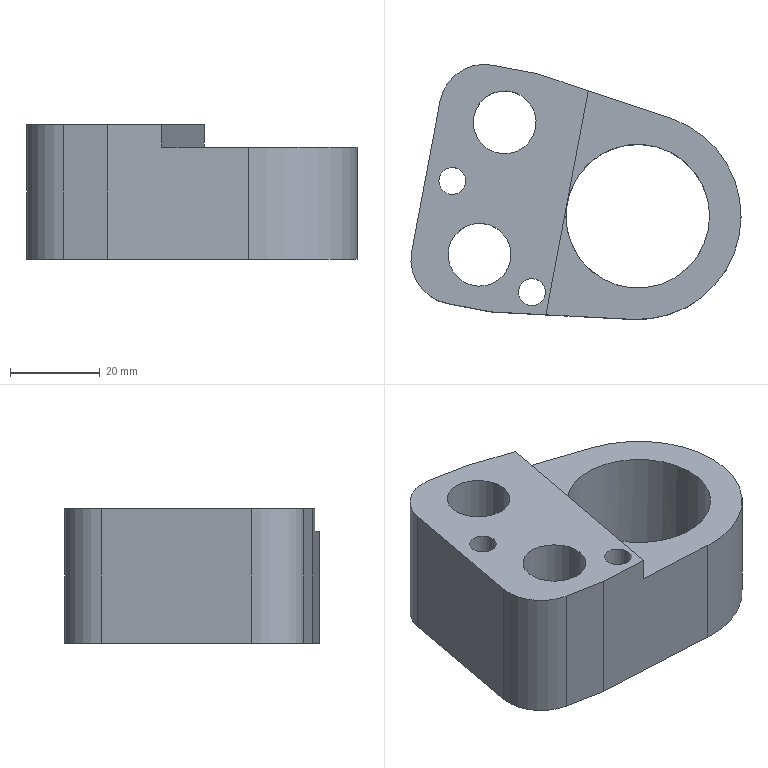Part | NX | features solid 2 | 1 solid | 25 faces | box 73.499 x 56.771 x 30 mm | volume 54639 mm3 | plane 13 | cylinder 12 | commonest cylinder face diameters 6 x2 8 x2 14 x2 19 x2 20 x2 32 x1
STEP:
#1=CARTESIAN_POINT('',(-713.065,445.332,68.));
#2=VERTEX_POINT('',#1);
#3=CARTESIAN_POINT('',(-716.996,446.076,68.));
#4=DIRECTION('',(0.,0.,1.));
#5=DIRECTION('',(0.9826,-0.186,0.));
#6=AXIS2_PLACEMENT_3D('',#3,#4,#5);
#7=CIRCLE('',#6,4.);
#8=EDGE_CURVE('',#2,#2,#7,.F.);
#9=ORIENTED_EDGE('',*,*,#8,.F.);
#10=EDGE_LOOP('',(#9));
#11=FACE_BOUND('',#10,.T.);
#12=CARTESIAN_POINT('',(-720.277,431.431,68.));
#13=VERTEX_POINT('',#12);
#14=CARTESIAN_POINT('',(-710.942,429.664,68.));
#15=DIRECTION('',(0.,0.,-1.));
#16=DIRECTION('',(-0.9826,0.186,0.));
#17=AXIS2_PLACEMENT_3D('',#14,#15,#16);
#18=CIRCLE('',#17,9.5);
#19=EDGE_CURVE('',#13,#13,#18,.T.);
#20=ORIENTED_EDGE('',*,*,#19,.F.);
#21=EDGE_LOOP('',(#20));
#22=FACE_BOUND('',#21,.T.);
#23=CARTESIAN_POINT('',(-714.697,460.908,68.));
#24=VERTEX_POINT('',#23);
#25=CARTESIAN_POINT('',(-705.363,459.141,68.));
#26=DIRECTION('',(0.,0.,-1.));
#27=DIRECTION('',(-0.9826,0.186,0.));
#28=AXIS2_PLACEMENT_3D('',#25,#26,#27);
#29=CIRCLE('',#28,9.5);
#30=EDGE_CURVE('',#24,#24,#29,.T.);
#31=ORIENTED_EDGE('',*,*,#30,.F.);
#32=EDGE_LOOP('',(#31));
#33=FACE_BOUND('',#32,.T.);
#34=CARTESIAN_POINT('',(-660.007,435.289,68.));
#35=VERTEX_POINT('',#34);
#36=CARTESIAN_POINT('',(-675.728,438.265,68.));
#37=DIRECTION('',(0.,0.,1.));
#38=DIRECTION('',(0.9826,-0.186,0.));
#39=AXIS2_PLACEMENT_3D('',#36,#37,#38);
#40=CIRCLE('',#39,16.);
#41=EDGE_CURVE('',#35,#35,#40,.T.);
#42=ORIENTED_EDGE('',*,*,#41,.T.);
#43=EDGE_LOOP('',(#42));
#44=FACE_BOUND('',#43,.T.);
#45=CARTESIAN_POINT('',(-668.458,460.086,68.));
#46=VERTEX_POINT('',#45);
#47=CARTESIAN_POINT('',(-698.218,470.002,68.));
#48=VERTEX_POINT('',#47);
#49=CARTESIAN_POINT('',(-668.458,460.086,68.));
#50=DIRECTION('',(-0.9487,0.3161,0.));
#51=VECTOR('',#50,1000.);
#52=LINE('',#49,#51);
#53=EDGE_CURVE('',#46,#48,#52,.T.);
#54=ORIENTED_EDGE('',*,*,#53,.F.);
#55=CARTESIAN_POINT('',(-676.936,415.297,68.));
#56=VERTEX_POINT('',#55);
#57=CARTESIAN_POINT('',(-675.728,438.265,68.));
#58=DIRECTION('',(0.,0.,-1.));
#59=DIRECTION('',(-0.9826,0.186,0.));
#60=AXIS2_PLACEMENT_3D('',#57,#58,#59);
#61=CIRCLE('',#60,23.);
#62=EDGE_CURVE('',#46,#56,#61,.T.);
#63=ORIENTED_EDGE('',*,*,#62,.T.);
#64=CARTESIAN_POINT('',(-708.261,416.944,68.));
#65=VERTEX_POINT('',#64);
#66=CARTESIAN_POINT('',(-676.936,415.297,68.));
#67=DIRECTION('',(-0.9986,0.0525,0.));
#68=VECTOR('',#67,1000.);
#69=LINE('',#66,#68);
#70=EDGE_CURVE('',#56,#65,#69,.T.);
#71=ORIENTED_EDGE('',*,*,#70,.T.);
#72=CARTESIAN_POINT('',(-718.087,418.804,68.));
#73=VERTEX_POINT('',#72);
#74=CARTESIAN_POINT('',(-708.261,416.944,68.));
#75=DIRECTION('',(-0.9826,0.186,0.));
#76=VECTOR('',#75,1000.);
#77=LINE('',#74,#76);
#78=EDGE_CURVE('',#65,#73,#77,.T.);
#79=ORIENTED_EDGE('',*,*,#78,.T.);
#80=CARTESIAN_POINT('',(-726.053,430.489,68.));
#81=VERTEX_POINT('',#80);
#82=CARTESIAN_POINT('',(-716.227,428.629,68.));
#83=DIRECTION('',(0.,0.,-1.));
#84=DIRECTION('',(-0.9826,0.186,0.));
#85=AXIS2_PLACEMENT_3D('',#82,#83,#84);
#86=CIRCLE('',#85,10.);
#87=EDGE_CURVE('',#73,#81,#86,.T.);
#88=ORIENTED_EDGE('',*,*,#87,.T.);
#89=CARTESIAN_POINT('',(-719.729,463.896,68.));
#90=VERTEX_POINT('',#89);
#91=CARTESIAN_POINT('',(-719.729,463.896,68.));
#92=DIRECTION('',(-0.186,-0.9826,0.));
#93=VECTOR('',#92,1000.);
#94=LINE('',#91,#93);
#95=EDGE_CURVE('',#90,#81,#94,.T.);
#96=ORIENTED_EDGE('',*,*,#95,.F.);
#97=CARTESIAN_POINT('',(-708.044,471.861,68.));
#98=VERTEX_POINT('',#97);
#99=CARTESIAN_POINT('',(-709.904,462.036,68.));
#100=DIRECTION('',(0.,0.,-1.));
#101=DIRECTION('',(-0.9826,0.186,0.));
#102=AXIS2_PLACEMENT_3D('',#99,#100,#101);
#103=CIRCLE('',#102,10.);
#104=EDGE_CURVE('',#90,#98,#103,.T.);
#105=ORIENTED_EDGE('',*,*,#104,.T.);
#106=CARTESIAN_POINT('',(-698.218,470.002,68.));
#107=DIRECTION('',(-0.9826,0.186,0.));
#108=VECTOR('',#107,1000.);
#109=LINE('',#106,#108);
#110=EDGE_CURVE('',#48,#98,#109,.T.);
#111=ORIENTED_EDGE('',*,*,#110,.F.);
#112=EDGE_LOOP('',(#54,#63,#71,#79,#88,#96,#105,#111));
#113=FACE_BOUND('',#112,.T.);
#114=CARTESIAN_POINT('',(-695.355,420.607,68.));
#115=VERTEX_POINT('',#114);
#116=CARTESIAN_POINT('',(-699.285,421.351,68.));
#117=DIRECTION('',(0.,0.,1.));
#118=DIRECTION('',(0.9826,-0.186,0.));
#119=AXIS2_PLACEMENT_3D('',#116,#117,#118);
#120=CIRCLE('',#119,4.);
#121=EDGE_CURVE('',#115,#115,#120,.F.);
#122=ORIENTED_EDGE('',*,*,#121,.F.);
#123=EDGE_LOOP('',(#122));
#124=FACE_BOUND('',#123,.T.);
#125=CARTESIAN_POINT('',(-709.904,462.036,68.));
#126=DIRECTION('',(0.,0.,-1.));
#127=DIRECTION('',(-0.9826,0.186,0.));
#128=AXIS2_PLACEMENT_3D('',#125,#126,#127);
#129=PLANE('',#128);
#130=ADVANCED_FACE('',(#11,#22,#33,#44,#113,#124),#129,.T.);
#131=CARTESIAN_POINT('',(-719.943,446.634,98.));
#132=VERTEX_POINT('',#131);
#133=CARTESIAN_POINT('',(-716.996,446.076,98.));
#134=DIRECTION('',(0.,0.,-1.));
#135=DIRECTION('',(-0.9826,0.186,0.));
#136=AXIS2_PLACEMENT_3D('',#133,#134,#135);
#137=CIRCLE('',#136,3.);
#138=EDGE_CURVE('',#132,#132,#137,.T.);
#139=ORIENTED_EDGE('',*,*,#138,.F.);
#140=EDGE_LOOP('',(#139));
#141=FACE_BOUND('',#140,.T.);
#142=CARTESIAN_POINT('',(-719.943,446.634,88.));
#143=VERTEX_POINT('',#142);
#144=CARTESIAN_POINT('',(-716.996,446.076,88.));
#145=DIRECTION('',(0.,0.,-1.));
#146=DIRECTION('',(-0.9826,0.186,0.));
#147=AXIS2_PLACEMENT_3D('',#144,#145,#146);
#148=CIRCLE('',#147,3.);
#149=EDGE_CURVE('',#143,#143,#148,.T.);
#150=ORIENTED_EDGE('',*,*,#149,.T.);
#151=EDGE_LOOP('',(#150));
#152=FACE_BOUND('',#151,.T.);
#153=CARTESIAN_POINT('',(-716.996,446.076,68.));
#154=DIRECTION('',(0.,0.,1.));
#155=DIRECTION('',(0.9826,-0.186,0.));
#156=AXIS2_PLACEMENT_3D('',#153,#154,#155);
#157=CYLINDRICAL_SURFACE('',#156,3.);
#158=ADVANCED_FACE('',(#141,#152),#157,.F.);
#159=CARTESIAN_POINT('',(-717.82,430.966,98.));
#160=VERTEX_POINT('',#159);
#161=CARTESIAN_POINT('',(-710.942,429.664,98.));
#162=DIRECTION('',(0.,0.,-1.));
#163=DIRECTION('',(-0.9826,0.186,0.));
#164=AXIS2_PLACEMENT_3D('',#161,#162,#163);
#165=CIRCLE('',#164,7.);
#166=EDGE_CURVE('',#160,#160,#165,.T.);
#167=ORIENTED_EDGE('',*,*,#166,.F.);
#168=EDGE_LOOP('',(#167));
#169=FACE_BOUND('',#168,.T.);
#170=CARTESIAN_POINT('',(-717.82,430.966,82.));
#171=VERTEX_POINT('',#170);
#172=CARTESIAN_POINT('',(-710.942,429.664,82.));
#173=DIRECTION('',(0.,0.,-1.));
#174=DIRECTION('',(-0.9826,0.186,0.));
#175=AXIS2_PLACEMENT_3D('',#172,#173,#174);
#176=CIRCLE('',#175,7.);
#177=EDGE_CURVE('',#171,#171,#176,.T.);
#178=ORIENTED_EDGE('',*,*,#177,.T.);
#179=EDGE_LOOP('',(#178));
#180=FACE_BOUND('',#179,.T.);
#181=CARTESIAN_POINT('',(-710.942,429.664,68.));
#182=DIRECTION('',(0.,0.,1.));
#183=DIRECTION('',(0.9826,-0.186,0.));
#184=AXIS2_PLACEMENT_3D('',#181,#182,#183);
#185=CYLINDRICAL_SURFACE('',#184,7.);
#186=ADVANCED_FACE('',(#169,#180),#185,.F.);
#187=CARTESIAN_POINT('',(-712.241,460.443,98.));
#188=VERTEX_POINT('',#187);
#189=CARTESIAN_POINT('',(-705.363,459.141,98.));
#190=DIRECTION('',(0.,0.,-1.));
#191=DIRECTION('',(-0.9826,0.186,0.));
#192=AXIS2_PLACEMENT_3D('',#189,#190,#191);
#193=CIRCLE('',#192,7.);
#194=EDGE_CURVE('',#188,#188,#193,.T.);
#195=ORIENTED_EDGE('',*,*,#194,.F.);
#196=EDGE_LOOP('',(#195));
#197=FACE_BOUND('',#196,.T.);
#198=CARTESIAN_POINT('',(-712.241,460.443,82.));
#199=VERTEX_POINT('',#198);
#200=CARTESIAN_POINT('',(-705.363,459.141,82.));
#201=DIRECTION('',(0.,0.,-1.));
#202=DIRECTION('',(-0.9826,0.186,0.));
#203=AXIS2_PLACEMENT_3D('',#200,#201,#202);
#204=CIRCLE('',#203,7.);
#205=EDGE_CURVE('',#199,#199,#204,.T.);
#206=ORIENTED_EDGE('',*,*,#205,.T.);
#207=EDGE_LOOP('',(#206));
#208=FACE_BOUND('',#207,.T.);
#209=CARTESIAN_POINT('',(-705.363,459.141,68.));
#210=DIRECTION('',(0.,0.,1.));
#211=DIRECTION('',(0.9826,-0.186,0.));
#212=AXIS2_PLACEMENT_3D('',#209,#210,#211);
#213=CYLINDRICAL_SURFACE('',#212,7.);
#214=ADVANCED_FACE('',(#197,#208),#213,.F.);
#215=CARTESIAN_POINT('',(-702.233,421.909,98.));
#216=VERTEX_POINT('',#215);
#217=CARTESIAN_POINT('',(-699.285,421.351,98.));
#218=DIRECTION('',(0.,0.,-1.));
#219=DIRECTION('',(-0.9826,0.186,0.));
#220=AXIS2_PLACEMENT_3D('',#217,#218,#219);
#221=CIRCLE('',#220,3.);
#222=EDGE_CURVE('',#216,#216,#221,.T.);
#223=ORIENTED_EDGE('',*,*,#222,.T.);
#224=EDGE_LOOP('',(#223));
#225=FACE_BOUND('',#224,.T.);
#226=ORIENTED_EDGE('',*,*,#166,.T.);
#227=EDGE_LOOP('',(#226));
#228=FACE_BOUND('',#227,.T.);
#229=CARTESIAN_POINT('',(-696.169,416.308,98.));
#230=VERTEX_POINT('',#229);
#231=CARTESIAN_POINT('',(-708.261,416.944,98.));
#232=VERTEX_POINT('',#231);
#233=CARTESIAN_POINT('',(-676.936,415.297,98.));
#234=DIRECTION('',(-0.9986,0.0525,0.));
#235=VECTOR('',#234,1000.);
#236=LINE('',#233,#235);
#237=EDGE_CURVE('',#230,#232,#236,.T.);
#238=ORIENTED_EDGE('',*,*,#237,.F.);
#239=CARTESIAN_POINT('',(-686.73,466.174,98.));
#240=VERTEX_POINT('',#239);
#241=CARTESIAN_POINT('',(-686.73,466.174,98.));
#242=DIRECTION('',(-0.186,-0.9826,0.));
#243=VECTOR('',#242,1000.);
#244=LINE('',#241,#243);
#245=EDGE_CURVE('',#240,#230,#244,.T.);
#246=ORIENTED_EDGE('',*,*,#245,.F.);
#247=CARTESIAN_POINT('',(-698.218,470.002,98.));
#248=VERTEX_POINT('',#247);
#249=CARTESIAN_POINT('',(-668.458,460.086,98.));
#250=DIRECTION('',(-0.9487,0.3161,0.));
#251=VECTOR('',#250,1000.);
#252=LINE('',#249,#251);
#253=EDGE_CURVE('',#240,#248,#252,.T.);
#254=ORIENTED_EDGE('',*,*,#253,.T.);
#255=CARTESIAN_POINT('',(-708.044,471.861,98.));
#256=VERTEX_POINT('',#255);
#257=CARTESIAN_POINT('',(-698.218,470.002,98.));
#258=DIRECTION('',(-0.9826,0.186,0.));
#259=VECTOR('',#258,1000.);
#260=LINE('',#257,#259);
#261=EDGE_CURVE('',#248,#256,#260,.T.);
#262=ORIENTED_EDGE('',*,*,#261,.T.);
#263=CARTESIAN_POINT('',(-719.729,463.896,98.));
#264=VERTEX_POINT('',#263);
#265=CARTESIAN_POINT('',(-709.904,462.036,98.));
#266=DIRECTION('',(0.,0.,-1.));
#267=DIRECTION('',(-0.9826,0.186,0.));
#268=AXIS2_PLACEMENT_3D('',#265,#266,#267);
#269=CIRCLE('',#268,10.);
#270=EDGE_CURVE('',#264,#256,#269,.T.);
#271=ORIENTED_EDGE('',*,*,#270,.F.);
#272=CARTESIAN_POINT('',(-726.053,430.489,98.));
#273=VERTEX_POINT('',#272);
#274=CARTESIAN_POINT('',(-719.729,463.896,98.));
#275=DIRECTION('',(-0.186,-0.9826,0.));
#276=VECTOR('',#275,1000.);
#277=LINE('',#274,#276);
#278=EDGE_CURVE('',#264,#273,#277,.T.);
#279=ORIENTED_EDGE('',*,*,#278,.T.);
#280=CARTESIAN_POINT('',(-718.087,418.804,98.));
#281=VERTEX_POINT('',#280);
#282=CARTESIAN_POINT('',(-716.227,428.629,98.));
#283=DIRECTION('',(0.,0.,-1.));
#284=DIRECTION('',(-0.9826,0.186,0.));
#285=AXIS2_PLACEMENT_3D('',#282,#283,#284);
#286=CIRCLE('',#285,10.);
#287=EDGE_CURVE('',#281,#273,#286,.T.);
#288=ORIENTED_EDGE('',*,*,#287,.F.);
#289=CARTESIAN_POINT('',(-708.261,416.944,98.));
#290=DIRECTION('',(-0.9826,0.186,0.));
#291=VECTOR('',#290,1000.);
#292=LINE('',#289,#291);
#293=EDGE_CURVE('',#232,#281,#292,.T.);
#294=ORIENTED_EDGE('',*,*,#293,.F.);
#295=EDGE_LOOP('',(#238,#246,#254,#262,#271,#279,#288,#294));
#296=FACE_BOUND('',#295,.T.);
#297=ORIENTED_EDGE('',*,*,#194,.T.);
#298=EDGE_LOOP('',(#297));
#299=FACE_BOUND('',#298,.T.);
#300=ORIENTED_EDGE('',*,*,#138,.T.);
#301=EDGE_LOOP('',(#300));
#302=FACE_BOUND('',#301,.T.);
#303=CARTESIAN_POINT('',(-709.904,462.036,98.));
#304=DIRECTION('',(0.,0.,-1.));
#305=DIRECTION('',(-0.9826,0.186,0.));
#306=AXIS2_PLACEMENT_3D('',#303,#304,#305);
#307=PLANE('',#306);
#308=ADVANCED_FACE('',(#225,#228,#296,#299,#302),#307,.F.);
#309=CARTESIAN_POINT('',(-686.73,466.174,93.));
#310=VERTEX_POINT('',#309);
#311=CARTESIAN_POINT('',(-686.73,466.174,93.));
#312=DIRECTION('',(0.,0.,1.));
#313=VECTOR('',#312,1000.);
#314=LINE('',#311,#313);
#315=EDGE_CURVE('',#310,#240,#314,.T.);
#316=ORIENTED_EDGE('',*,*,#315,.F.);
#317=CARTESIAN_POINT('',(-668.458,460.086,93.));
#318=VERTEX_POINT('',#317);
#319=CARTESIAN_POINT('',(-686.73,466.174,93.));
#320=DIRECTION('',(0.9487,-0.3161,0.));
#321=VECTOR('',#320,1000.);
#322=LINE('',#319,#321);
#323=EDGE_CURVE('',#310,#318,#322,.T.);
#324=ORIENTED_EDGE('',*,*,#323,.T.);
#325=CARTESIAN_POINT('',(-668.458,460.086,68.));
#326=DIRECTION('',(0.,0.,1.));
#327=VECTOR('',#326,1000.);
#328=LINE('',#325,#327);
#329=EDGE_CURVE('',#46,#318,#328,.T.);
#330=ORIENTED_EDGE('',*,*,#329,.F.);
#331=ORIENTED_EDGE('',*,*,#53,.T.);
#332=CARTESIAN_POINT('',(-698.218,470.002,68.));
#333=DIRECTION('',(0.,0.,1.));
#334=VECTOR('',#333,1000.);
#335=LINE('',#332,#334);
#336=EDGE_CURVE('',#48,#248,#335,.T.);
#337=ORIENTED_EDGE('',*,*,#336,.T.);
#338=ORIENTED_EDGE('',*,*,#253,.F.);
#339=EDGE_LOOP('',(#316,#324,#330,#331,#337,#338));
#340=FACE_BOUND('',#339,.T.);
#341=CARTESIAN_POINT('',(-668.458,460.086,68.));
#342=DIRECTION('',(0.3161,0.9487,0.));
#343=DIRECTION('',(-0.9487,0.3161,0.));
#344=AXIS2_PLACEMENT_3D('',#341,#342,#343);
#345=PLANE('',#344);
#346=ADVANCED_FACE('',(#340),#345,.T.);
#347=ORIENTED_EDGE('',*,*,#261,.F.);
#348=ORIENTED_EDGE('',*,*,#336,.F.);
#349=ORIENTED_EDGE('',*,*,#110,.T.);
#350=CARTESIAN_POINT('',(-708.044,471.861,68.));
#351=DIRECTION('',(0.,0.,1.));
#352=VECTOR('',#351,1000.);
#353=LINE('',#350,#352);
#354=EDGE_CURVE('',#98,#256,#353,.T.);
#355=ORIENTED_EDGE('',*,*,#354,.T.);
#356=EDGE_LOOP('',(#347,#348,#349,#355));
#357=FACE_BOUND('',#356,.T.);
#358=CARTESIAN_POINT('',(-698.218,470.002,68.));
#359=DIRECTION('',(0.186,0.9826,0.));
#360=DIRECTION('',(-0.9826,0.186,0.));
#361=AXIS2_PLACEMENT_3D('',#358,#359,#360);
#362=PLANE('',#361);
#363=ADVANCED_FACE('',(#357),#362,.T.);
#364=ORIENTED_EDGE('',*,*,#270,.T.);
#365=ORIENTED_EDGE('',*,*,#354,.F.);
#366=ORIENTED_EDGE('',*,*,#104,.F.);
#367=CARTESIAN_POINT('',(-719.729,463.896,68.));
#368=DIRECTION('',(0.,0.,1.));
#369=VECTOR('',#368,1000.);
#370=LINE('',#367,#369);
#371=EDGE_CURVE('',#90,#264,#370,.T.);
#372=ORIENTED_EDGE('',*,*,#371,.T.);
#373=EDGE_LOOP('',(#364,#365,#366,#372));
#374=FACE_BOUND('',#373,.T.);
#375=CARTESIAN_POINT('',(-709.904,462.036,68.));
#376=DIRECTION('',(0.,0.,1.));
#377=DIRECTION('',(0.9826,-0.186,0.));
#378=AXIS2_PLACEMENT_3D('',#375,#376,#377);
#379=CYLINDRICAL_SURFACE('',#378,10.);
#380=ADVANCED_FACE('',(#374),#379,.T.);
#381=ORIENTED_EDGE('',*,*,#278,.F.);
#382=ORIENTED_EDGE('',*,*,#371,.F.);
#383=ORIENTED_EDGE('',*,*,#95,.T.);
#384=CARTESIAN_POINT('',(-726.053,430.489,68.));
#385=DIRECTION('',(0.,0.,1.));
#386=VECTOR('',#385,1000.);
#387=LINE('',#384,#386);
#388=EDGE_CURVE('',#81,#273,#387,.T.);
#389=ORIENTED_EDGE('',*,*,#388,.T.);
#390=EDGE_LOOP('',(#381,#382,#383,#389));
#391=FACE_BOUND('',#390,.T.);
#392=CARTESIAN_POINT('',(-719.729,463.896,68.));
#393=DIRECTION('',(-0.9826,0.186,0.));
#394=DIRECTION('',(-0.186,-0.9826,0.));
#395=AXIS2_PLACEMENT_3D('',#392,#393,#394);
#396=PLANE('',#395);
#397=ADVANCED_FACE('',(#391),#396,.T.);
#398=ORIENTED_EDGE('',*,*,#287,.T.);
#399=ORIENTED_EDGE('',*,*,#388,.F.);
#400=ORIENTED_EDGE('',*,*,#87,.F.);
#401=CARTESIAN_POINT('',(-718.087,418.804,68.));
#402=DIRECTION('',(0.,0.,1.));
#403=VECTOR('',#402,1000.);
#404=LINE('',#401,#403);
#405=EDGE_CURVE('',#73,#281,#404,.T.);
#406=ORIENTED_EDGE('',*,*,#405,.T.);
#407=EDGE_LOOP('',(#398,#399,#400,#406));
#408=FACE_BOUND('',#407,.T.);
#409=CARTESIAN_POINT('',(-716.227,428.629,68.));
#410=DIRECTION('',(0.,0.,1.));
#411=DIRECTION('',(0.9826,-0.186,0.));
#412=AXIS2_PLACEMENT_3D('',#409,#410,#411);
#413=CYLINDRICAL_SURFACE('',#412,10.);
#414=ADVANCED_FACE('',(#408),#413,.T.);
#415=ORIENTED_EDGE('',*,*,#293,.T.);
#416=ORIENTED_EDGE('',*,*,#405,.F.);
#417=ORIENTED_EDGE('',*,*,#78,.F.);
#418=CARTESIAN_POINT('',(-708.261,416.944,68.));
#419=DIRECTION('',(0.,0.,1.));
#420=VECTOR('',#419,1000.);
#421=LINE('',#418,#420);
#422=EDGE_CURVE('',#65,#232,#421,.T.);
#423=ORIENTED_EDGE('',*,*,#422,.T.);
#424=EDGE_LOOP('',(#415,#416,#417,#423));
#425=FACE_BOUND('',#424,.T.);
#426=CARTESIAN_POINT('',(-708.261,416.944,68.));
#427=DIRECTION('',(0.186,0.9826,0.));
#428=DIRECTION('',(-0.9826,0.186,0.));
#429=AXIS2_PLACEMENT_3D('',#426,#427,#428);
#430=PLANE('',#429);
#431=ADVANCED_FACE('',(#425),#430,.F.);
#432=CARTESIAN_POINT('',(-696.169,416.308,93.));
#433=VERTEX_POINT('',#432);
#434=CARTESIAN_POINT('',(-676.936,415.297,93.));
#435=VERTEX_POINT('',#434);
#436=CARTESIAN_POINT('',(-696.169,416.308,93.));
#437=DIRECTION('',(0.9986,-0.0525,0.));
#438=VECTOR('',#437,1000.);
#439=LINE('',#436,#438);
#440=EDGE_CURVE('',#433,#435,#439,.T.);
#441=ORIENTED_EDGE('',*,*,#440,.F.);
#442=CARTESIAN_POINT('',(-696.169,416.308,93.));
#443=DIRECTION('',(0.,0.,1.));
#444=VECTOR('',#443,1000.);
#445=LINE('',#442,#444);
#446=EDGE_CURVE('',#433,#230,#445,.T.);
#447=ORIENTED_EDGE('',*,*,#446,.T.);
#448=ORIENTED_EDGE('',*,*,#237,.T.);
#449=ORIENTED_EDGE('',*,*,#422,.F.);
#450=ORIENTED_EDGE('',*,*,#70,.F.);
#451=CARTESIAN_POINT('',(-676.936,415.297,68.));
#452=DIRECTION('',(0.,0.,1.));
#453=VECTOR('',#452,1000.);
#454=LINE('',#451,#453);
#455=EDGE_CURVE('',#56,#435,#454,.T.);
#456=ORIENTED_EDGE('',*,*,#455,.T.);
#457=EDGE_LOOP('',(#441,#447,#448,#449,#450,#456));
#458=FACE_BOUND('',#457,.T.);
#459=CARTESIAN_POINT('',(-676.936,415.297,68.));
#460=DIRECTION('',(0.0525,0.9986,0.));
#461=DIRECTION('',(-0.9986,0.0525,0.));
#462=AXIS2_PLACEMENT_3D('',#459,#460,#461);
#463=PLANE('',#462);
#464=ADVANCED_FACE('',(#458),#463,.F.);
#465=ORIENTED_EDGE('',*,*,#329,.T.);
#466=CARTESIAN_POINT('',(-675.728,438.265,93.));
#467=DIRECTION('',(0.,0.,-1.));
#468=DIRECTION('',(-0.9826,0.186,0.));
#469=AXIS2_PLACEMENT_3D('',#466,#467,#468);
#470=CIRCLE('',#469,23.);
#471=EDGE_CURVE('',#318,#435,#470,.T.);
#472=ORIENTED_EDGE('',*,*,#471,.T.);
#473=ORIENTED_EDGE('',*,*,#455,.F.);
#474=ORIENTED_EDGE('',*,*,#62,.F.);
#475=EDGE_LOOP('',(#465,#472,#473,#474));
#476=FACE_BOUND('',#475,.T.);
#477=CARTESIAN_POINT('',(-675.728,438.265,68.));
#478=DIRECTION('',(0.,0.,1.));
#479=DIRECTION('',(0.9826,-0.186,0.));
#480=AXIS2_PLACEMENT_3D('',#477,#478,#479);
#481=CYLINDRICAL_SURFACE('',#480,23.);
#482=ADVANCED_FACE('',(#476),#481,.T.);
#483=CARTESIAN_POINT('',(-691.449,441.241,93.));
#484=VERTEX_POINT('',#483);
#485=CARTESIAN_POINT('',(-675.728,438.265,93.));
#486=DIRECTION('',(0.,0.,-1.));
#487=DIRECTION('',(-0.9826,0.186,0.));
#488=AXIS2_PLACEMENT_3D('',#485,#486,#487);
#489=CIRCLE('',#488,16.);
#490=EDGE_CURVE('',#484,#484,#489,.F.);
#491=ORIENTED_EDGE('',*,*,#490,.T.);
#492=EDGE_LOOP('',(#491));
#493=FACE_BOUND('',#492,.T.);
#494=ORIENTED_EDGE('',*,*,#41,.F.);
#495=EDGE_LOOP('',(#494));
#496=FACE_BOUND('',#495,.T.);
#497=CARTESIAN_POINT('',(-675.728,438.265,68.));
#498=DIRECTION('',(0.,0.,1.));
#499=DIRECTION('',(0.9826,-0.186,0.));
#500=AXIS2_PLACEMENT_3D('',#497,#498,#499);
#501=CYLINDRICAL_SURFACE('',#500,16.);
#502=ADVANCED_FACE('',(#493,#496),#501,.F.);
#503=ORIENTED_EDGE('',*,*,#245,.T.);
#504=ORIENTED_EDGE('',*,*,#446,.F.);
#505=CARTESIAN_POINT('',(-686.73,466.174,93.));
#506=DIRECTION('',(-0.186,-0.9826,0.));
#507=VECTOR('',#506,1000.);
#508=LINE('',#505,#507);
#509=EDGE_CURVE('',#484,#433,#508,.T.);
#510=ORIENTED_EDGE('',*,*,#509,.F.);
#511=CARTESIAN_POINT('',(-686.73,466.174,93.));
#512=DIRECTION('',(-0.186,-0.9826,0.));
#513=VECTOR('',#512,1000.);
#514=LINE('',#511,#513);
#515=EDGE_CURVE('',#310,#484,#514,.T.);
#516=ORIENTED_EDGE('',*,*,#515,.F.);
#517=ORIENTED_EDGE('',*,*,#315,.T.);
#518=EDGE_LOOP('',(#503,#504,#510,#516,#517));
#519=FACE_BOUND('',#518,.T.);
#520=CARTESIAN_POINT('',(-686.73,466.174,93.));
#521=DIRECTION('',(-0.9826,0.186,0.));
#522=DIRECTION('',(-0.186,-0.9826,0.));
#523=AXIS2_PLACEMENT_3D('',#520,#521,#522);
#524=PLANE('',#523);
#525=ADVANCED_FACE('',(#519),#524,.F.);
#526=ORIENTED_EDGE('',*,*,#509,.T.);
#527=ORIENTED_EDGE('',*,*,#440,.T.);
#528=ORIENTED_EDGE('',*,*,#471,.F.);
#529=ORIENTED_EDGE('',*,*,#323,.F.);
#530=ORIENTED_EDGE('',*,*,#515,.T.);
#531=ORIENTED_EDGE('',*,*,#490,.F.);
#532=EDGE_LOOP('',(#526,#527,#528,#529,#530,#531));
#533=FACE_BOUND('',#532,.T.);
#534=CARTESIAN_POINT('',(-675.728,438.265,93.));
#535=DIRECTION('',(0.,0.,-1.));
#536=DIRECTION('',(-0.9826,0.186,0.));
#537=AXIS2_PLACEMENT_3D('',#534,#535,#536);
#538=PLANE('',#537);
#539=ADVANCED_FACE('',(#533),#538,.F.);
#540=CARTESIAN_POINT('',(-702.233,421.909,88.));
#541=VERTEX_POINT('',#540);
#542=CARTESIAN_POINT('',(-699.285,421.351,88.));
#543=DIRECTION('',(0.,0.,-1.));
#544=DIRECTION('',(-0.9826,0.186,0.));
#545=AXIS2_PLACEMENT_3D('',#542,#543,#544);
#546=CIRCLE('',#545,3.);
#547=EDGE_CURVE('',#541,#541,#546,.T.);
#548=ORIENTED_EDGE('',*,*,#547,.T.);
#549=EDGE_LOOP('',(#548));
#550=FACE_BOUND('',#549,.T.);
#551=ORIENTED_EDGE('',*,*,#222,.F.);
#552=EDGE_LOOP('',(#551));
#553=FACE_BOUND('',#552,.T.);
#554=CARTESIAN_POINT('',(-699.285,421.351,68.));
#555=DIRECTION('',(0.,0.,1.));
#556=DIRECTION('',(0.9826,-0.186,0.));
#557=AXIS2_PLACEMENT_3D('',#554,#555,#556);
#558=CYLINDRICAL_SURFACE('',#557,3.);
#559=ADVANCED_FACE('',(#550,#553),#558,.F.);
#560=CARTESIAN_POINT('',(-714.697,460.908,82.));
#561=VERTEX_POINT('',#560);
#562=CARTESIAN_POINT('',(-705.363,459.141,82.));
#563=DIRECTION('',(0.,0.,-1.));
#564=DIRECTION('',(-0.9826,0.186,0.));
#565=AXIS2_PLACEMENT_3D('',#562,#563,#564);
#566=CIRCLE('',#565,9.5);
#567=EDGE_CURVE('',#561,#561,#566,.T.);
#568=ORIENTED_EDGE('',*,*,#567,.F.);
#569=EDGE_LOOP('',(#568));
#570=FACE_BOUND('',#569,.T.);
#571=ORIENTED_EDGE('',*,*,#30,.T.);
#572=EDGE_LOOP('',(#571));
#573=FACE_BOUND('',#572,.T.);
#574=CARTESIAN_POINT('',(-705.363,459.141,82.));
#575=DIRECTION('',(0.,0.,-1.));
#576=DIRECTION('',(-0.9826,0.186,0.));
#577=AXIS2_PLACEMENT_3D('',#574,#575,#576);
#578=CYLINDRICAL_SURFACE('',#577,9.5);
#579=ADVANCED_FACE('',(#570,#573),#578,.F.);
#580=ORIENTED_EDGE('',*,*,#205,.F.);
#581=EDGE_LOOP('',(#580));
#582=FACE_BOUND('',#581,.T.);
#583=ORIENTED_EDGE('',*,*,#567,.T.);
#584=EDGE_LOOP('',(#583));
#585=FACE_BOUND('',#584,.T.);
#586=CARTESIAN_POINT('',(-705.363,459.141,82.));
#587=DIRECTION('',(0.,0.,-1.));
#588=DIRECTION('',(-0.9826,0.186,0.));
#589=AXIS2_PLACEMENT_3D('',#586,#587,#588);
#590=PLANE('',#589);
#591=ADVANCED_FACE('',(#582,#585),#590,.T.);
#592=CARTESIAN_POINT('',(-720.277,431.431,82.));
#593=VERTEX_POINT('',#592);
#594=CARTESIAN_POINT('',(-710.942,429.664,82.));
#595=DIRECTION('',(0.,0.,-1.));
#596=DIRECTION('',(-0.9826,0.186,0.));
#597=AXIS2_PLACEMENT_3D('',#594,#595,#596);
#598=CIRCLE('',#597,9.5);
#599=EDGE_CURVE('',#593,#593,#598,.T.);
#600=ORIENTED_EDGE('',*,*,#599,.F.);
#601=EDGE_LOOP('',(#600));
#602=FACE_BOUND('',#601,.T.);
#603=ORIENTED_EDGE('',*,*,#19,.T.);
#604=EDGE_LOOP('',(#603));
#605=FACE_BOUND('',#604,.T.);
#606=CARTESIAN_POINT('',(-710.942,429.664,82.));
#607=DIRECTION('',(0.,0.,-1.));
#608=DIRECTION('',(-0.9826,0.186,0.));
#609=AXIS2_PLACEMENT_3D('',#606,#607,#608);
#610=CYLINDRICAL_SURFACE('',#609,9.5);
#611=ADVANCED_FACE('',(#602,#605),#610,.F.);
#612=ORIENTED_EDGE('',*,*,#177,.F.);
#613=EDGE_LOOP('',(#612));
#614=FACE_BOUND('',#613,.T.);
#615=ORIENTED_EDGE('',*,*,#599,.T.);
#616=EDGE_LOOP('',(#615));
#617=FACE_BOUND('',#616,.T.);
#618=CARTESIAN_POINT('',(-710.942,429.664,82.));
#619=DIRECTION('',(0.,0.,-1.));
#620=DIRECTION('',(-0.9826,0.186,0.));
#621=AXIS2_PLACEMENT_3D('',#618,#619,#620);
#622=PLANE('',#621);
#623=ADVANCED_FACE('',(#614,#617),#622,.T.);
#624=ORIENTED_EDGE('',*,*,#149,.F.);
#625=EDGE_LOOP('',(#624));
#626=FACE_BOUND('',#625,.T.);
#627=CARTESIAN_POINT('',(-713.065,445.332,88.));
#628=VERTEX_POINT('',#627);
#629=CARTESIAN_POINT('',(-716.996,446.076,88.));
#630=DIRECTION('',(0.,0.,1.));
#631=DIRECTION('',(0.9826,-0.186,0.));
#632=AXIS2_PLACEMENT_3D('',#629,#630,#631);
#633=CIRCLE('',#632,4.);
#634=EDGE_CURVE('',#628,#628,#633,.F.);
#635=ORIENTED_EDGE('',*,*,#634,.T.);
#636=EDGE_LOOP('',(#635));
#637=FACE_BOUND('',#636,.T.);
#638=CARTESIAN_POINT('',(-716.996,446.076,88.));
#639=DIRECTION('',(0.,0.,1.));
#640=DIRECTION('',(0.9826,-0.186,0.));
#641=AXIS2_PLACEMENT_3D('',#638,#639,#640);
#642=PLANE('',#641);
#643=ADVANCED_FACE('',(#626,#637),#642,.F.);
#644=ORIENTED_EDGE('',*,*,#634,.F.);
#645=EDGE_LOOP('',(#644));
#646=FACE_BOUND('',#645,.T.);
#647=ORIENTED_EDGE('',*,*,#8,.T.);
#648=EDGE_LOOP('',(#647));
#649=FACE_BOUND('',#648,.T.);
#650=CARTESIAN_POINT('',(-716.996,446.076,68.));
#651=DIRECTION('',(0.,0.,1.));
#652=DIRECTION('',(0.9826,-0.186,0.));
#653=AXIS2_PLACEMENT_3D('',#650,#651,#652);
#654=CYLINDRICAL_SURFACE('',#653,4.);
#655=ADVANCED_FACE('',(#646,#649),#654,.F.);
#656=ORIENTED_EDGE('',*,*,#547,.F.);
#657=EDGE_LOOP('',(#656));
#658=FACE_BOUND('',#657,.T.);
#659=CARTESIAN_POINT('',(-695.355,420.607,88.));
#660=VERTEX_POINT('',#659);
#661=CARTESIAN_POINT('',(-699.285,421.351,88.));
#662=DIRECTION('',(0.,0.,1.));
#663=DIRECTION('',(0.9826,-0.186,0.));
#664=AXIS2_PLACEMENT_3D('',#661,#662,#663);
#665=CIRCLE('',#664,4.);
#666=EDGE_CURVE('',#660,#660,#665,.F.);
#667=ORIENTED_EDGE('',*,*,#666,.T.);
#668=EDGE_LOOP('',(#667));
#669=FACE_BOUND('',#668,.T.);
#670=CARTESIAN_POINT('',(-699.285,421.351,88.));
#671=DIRECTION('',(0.,0.,1.));
#672=DIRECTION('',(0.9826,-0.186,0.));
#673=AXIS2_PLACEMENT_3D('',#670,#671,#672);
#674=PLANE('',#673);
#675=ADVANCED_FACE('',(#658,#669),#674,.F.);
#676=ORIENTED_EDGE('',*,*,#666,.F.);
#677=EDGE_LOOP('',(#676));
#678=FACE_BOUND('',#677,.T.);
#679=ORIENTED_EDGE('',*,*,#121,.T.);
#680=EDGE_LOOP('',(#679));
#681=FACE_BOUND('',#680,.T.);
#682=CARTESIAN_POINT('',(-699.285,421.351,68.));
#683=DIRECTION('',(0.,0.,1.));
#684=DIRECTION('',(0.9826,-0.186,0.));
#685=AXIS2_PLACEMENT_3D('',#682,#683,#684);
#686=CYLINDRICAL_SURFACE('',#685,4.);
#687=ADVANCED_FACE('',(#678,#681),#686,.F.);
#688=CLOSED_SHELL('',(#130,#158,#186,#214,#308,#346,#363,#380,#397,#414,#431,#464,#482,#502,#525,#539,#559,#579,#591,#611,#623,#643,#655,#675,#687));
#689=MANIFOLD_SOLID_BREP('',#688);
#690=(LENGTH_UNIT()NAMED_UNIT(*)SI_UNIT(.MILLI.,.METRE.));
#691=UNCERTAINTY_MEASURE_WITH_UNIT(LENGTH_MEASURE(0.00001),#690,'','');
#692=(NAMED_UNIT(*)PLANE_ANGLE_UNIT()SI_UNIT($,.RADIAN.));
#693=(NAMED_UNIT(*)SI_UNIT($,.STERADIAN.)SOLID_ANGLE_UNIT());
#694=(GEOMETRIC_REPRESENTATION_CONTEXT(3)GLOBAL_UNCERTAINTY_ASSIGNED_CONTEXT((#691))GLOBAL_UNIT_ASSIGNED_CONTEXT((#690,#692,#693))REPRESENTATION_CONTEXT('',''));
#695=ADVANCED_BREP_SHAPE_REPRESENTATION('',(#689),#694);